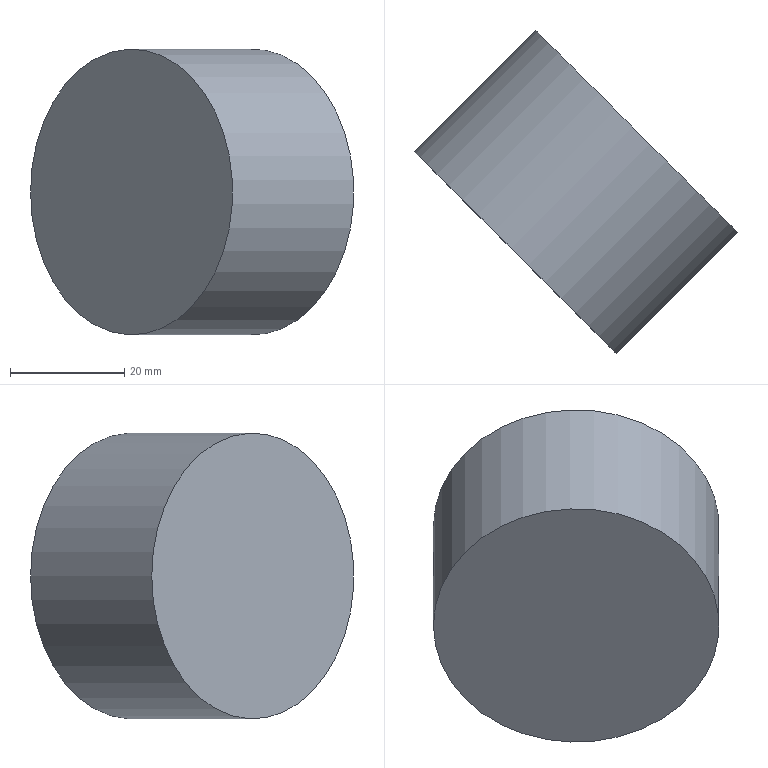Part | NX | features solid 2 | 1 solid | 3 faces | box 56.569 x 56.569 x 50 mm | volume 58905 mm3 | plane 2 | cylinder 1 | commonest cylinder face diameters 50 x1
STEP:
#1=CARTESIAN_POINT('',(784.889,-593.97,-50.));
#2=VERTEX_POINT('',#1);
#3=CARTESIAN_POINT('',(802.566,-611.647,-50.));
#4=DIRECTION('',(0.7071,0.7071,0.));
#5=DIRECTION('',(-0.7071,0.7071,0.));
#6=AXIS2_PLACEMENT_3D('',#3,#4,#5);
#7=CIRCLE('',#6,25.);
#8=EDGE_CURVE('',#2,#2,#7,.T.);
#9=ORIENTED_EDGE('',*,*,#8,.T.);
#10=EDGE_LOOP('',(#9));
#11=FACE_BOUND('',#10,.T.);
#12=CARTESIAN_POINT('',(806.102,-572.756,-50.));
#13=VERTEX_POINT('',#12);
#14=CARTESIAN_POINT('',(823.779,-590.434,-50.));
#15=DIRECTION('',(0.7071,0.7071,0.));
#16=DIRECTION('',(-0.7071,0.7071,0.));
#17=AXIS2_PLACEMENT_3D('',#14,#15,#16);
#18=CIRCLE('',#17,25.);
#19=EDGE_CURVE('',#13,#13,#18,.T.);
#20=ORIENTED_EDGE('',*,*,#19,.F.);
#21=EDGE_LOOP('',(#20));
#22=FACE_BOUND('',#21,.T.);
#23=CARTESIAN_POINT('',(802.566,-611.647,-50.));
#24=DIRECTION('',(0.7071,0.7071,0.));
#25=DIRECTION('',(0.,0.,-1.));
#26=AXIS2_PLACEMENT_3D('',#23,#24,#25);
#27=CYLINDRICAL_SURFACE('',#26,25.);
#28=ADVANCED_FACE('',(#11,#22),#27,.T.);
#29=ORIENTED_EDGE('',*,*,#8,.F.);
#30=EDGE_LOOP('',(#29));
#31=FACE_BOUND('',#30,.T.);
#32=CARTESIAN_POINT('',(802.566,-611.647,-50.));
#33=DIRECTION('',(0.7071,0.7071,0.));
#34=DIRECTION('',(0.,0.,-1.));
#35=AXIS2_PLACEMENT_3D('',#32,#33,#34);
#36=PLANE('',#35);
#37=ADVANCED_FACE('',(#31),#36,.F.);
#38=ORIENTED_EDGE('',*,*,#19,.T.);
#39=EDGE_LOOP('',(#38));
#40=FACE_BOUND('',#39,.T.);
#41=CARTESIAN_POINT('',(823.779,-590.434,-50.));
#42=DIRECTION('',(0.7071,0.7071,0.));
#43=DIRECTION('',(0.,0.,-1.));
#44=AXIS2_PLACEMENT_3D('',#41,#42,#43);
#45=PLANE('',#44);
#46=ADVANCED_FACE('',(#40),#45,.T.);
#47=CLOSED_SHELL('',(#28,#37,#46));
#48=MANIFOLD_SOLID_BREP('',#47);
#49=(LENGTH_UNIT()NAMED_UNIT(*)SI_UNIT(.MILLI.,.METRE.));
#50=UNCERTAINTY_MEASURE_WITH_UNIT(LENGTH_MEASURE(0.00001),#49,'','');
#51=(NAMED_UNIT(*)PLANE_ANGLE_UNIT()SI_UNIT($,.RADIAN.));
#52=(NAMED_UNIT(*)SI_UNIT($,.STERADIAN.)SOLID_ANGLE_UNIT());
#53=(GEOMETRIC_REPRESENTATION_CONTEXT(3)GLOBAL_UNCERTAINTY_ASSIGNED_CONTEXT((#50))GLOBAL_UNIT_ASSIGNED_CONTEXT((#49,#51,#52))REPRESENTATION_CONTEXT('',''));
#54=ADVANCED_BREP_SHAPE_REPRESENTATION('',(#48),#53);